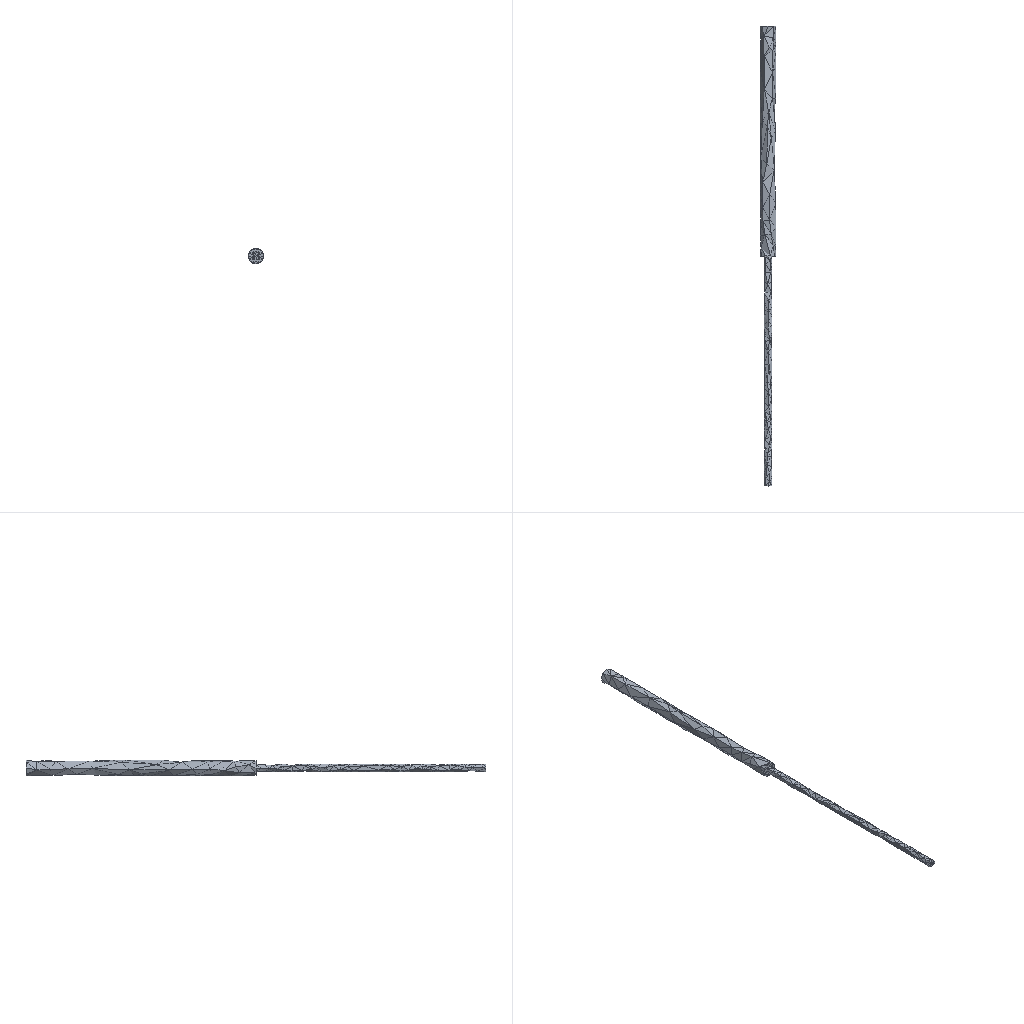Simulation study | ansys workbench
Ansys APDL input file, long lists of numbers shortened:
/batch
/config,noeldb,1     ! force off writing results to database
*get,_wallstrt,active,,time,wall
! ANSYS input file written by Workbench version 2022 R1
! File used for geometry attach: F:\ansys（分析文件汇总)\ansys有限元题目分析\1_files\dp0\SYS-1\DM\SYS-1.scdoc
/title,1--____ (B5)
! ****** Begin Custom Load Command Snippet ******
/COM, ACT Extensions:
/COM,     LSDYNA, 2021.1
/COM,
! ****** End   Custom Load Command Snippet ******
*DIM,_wb_ProjectScratch_dir,string,248
_wb_ProjectScratch_dir(1) = 'F:\ansys（分析文件汇总)\ansys有限元题目分析\_ProjectScratch\Scr897A\'
*DIM,_wb_SolverFiles_dir,string,248
_wb_SolverFiles_dir(1) = 'F:\ansys（分析文件汇总)\ansys有限元题目分析\1_files\dp0\SYS-1\MECH\'
*DIM,_wb_userfiles_dir,string,248
_wb_userfiles_dir(1) = 'F:\ansys（分析文件汇总)\ansys有限元题目分析\1_files\user_files\'
/com,--- Data in consistent NMM units. See Solving Units in the help system for more information.
/units,MPA
/nopr
/wb,file,start              !  signify a WB generated input file
/prep7
! Turn off shape checking because checks already performed inside WB mesher.
! See help system for more information.
SHPP,OFF,,NOWARN
/nolist
etcon,set             ! allow ANSYS to choose best KEYOP's for 180x elements, resets any applicable keyopt to MAPDL defaults
/com,*********** Nodes for the whole assembly ***********
nblock,3,,134372
(1i9,3e20.9e3)
        1    -5.000000000E+01     4.405700000E+02    -2.832769449E-14
! (122156 more lines like these left out)
-1
/com,*********** Nodes for all Remote Points ***********
nblock,3
(1i9,3e20.9e3)
   122158     1.673250921E-03     0.000000000E+00     1.798580280E-16
   122159    -8.638767374E-16     4.405699968E+02     2.339666164E-16
   122160     1.382202767E-15     9.615300298E+02     2.159691824E-16
-1
/wb,elem,start            !  set before creation of elements
/com,*********** Elements for Body 1 "SYS-1\__" ***********
et,1,187
eblock,19,solid,,70267
(19i9)
        1        1        1        1        0        0        0        0       10        0        1     9167     9394    19171    19168    69793    71048    69798    69797
! (140533 more lines like these left out)
-1
/wb,elem,end               !  done creating elements
/com,*********** Send User Defined Coordinate System(s) ***********
csys,0
toffst,273.15,  ! Temperature offset from absolute zero
/com,*********** Set Reference Temperature ***********
tref,22.
/wb,mat,start              !  starting to send materials
/com,*********** Send Materials ***********
Temperature = 'TEMP' ! Temperature
MP,DENS,1,7.85e-09,	! tonne mm^-3
MP,ALPX,1,1.2e-05,	! C^-1
MP,C,1,434000000,	! mm^2 s^-2 C^-1
MP,KXX,1,60.5,	! tonne mm s^-3 C^-1
MP,RSVX,1,0.00017,	! ohm mm
MP,EX,1,200000,	! tonne s^-2 mm^-1
MP,NUXY,1,0.3,
MP,MURX,1,10000,
/wb,mat,end                !  done sending materials
!************************* Model Summary ********************
!SYS-1\__,	结构钢,	matid,	1
!************************* End Model Summary ********************
! get the diagonal of the bounding box. Needed later for other things
*get,_xmin,node,,mnloc,x
*get,_ymin,node,,mnloc,y
*get,_zmin,node,,mnloc,z
*get,_xmax,node,,mxloc,x
*get,_ymax,node,,mxloc,y
*get,_zmax,node,,mxloc,z
_ASMDIAG=(_xmax-_xmin)*(_xmax-_xmin)+(_ymax-_ymin)*(_ymax-_ymin)+(_zmax-_zmin)*(_zmax-_zmin)
_ASMDIAG=SQRT(_ASMDIAG)
/wb,contact,start          !  starting to send contact
/wb,contact,end            !  done creating contacts
/golist
/wb,load,start             !  starting to send loads
/com,*********** Fixed Supports ***********
CMBLOCK,_FIXEDSU,NODE,     1223
(8i10)
        64        65        66        67        68        69        70        71
! (152 more lines like these left out)
cmsel,s,_FIXEDSU
d,all,all
nsel,all
/com,*********** Create Remote Point "内部远程点" ***********
! -------- Remote Point Used by "力矩" --------
*set,tid,3
*set,cid,2
et,cid,177
et,tid,170
keyo,tid,2,1               ! Don't fix the pilot node
keyo,tid,4,111111
keyo,cid,12,5              ! Bonded Contact
keyo,cid,4,1               ! Deformable RBE3 style load
keyo,cid,2,2               ! MPC style contact
eblock,10,,,76
(15i9)
    97369        2        2        2        0      204      203    20501
! (75 more lines like these left out)
-1
*set,_npilot,122158
_npilot33=_npilot
type,tid
mat ,cid
real,cid
tshape,pilo
en,97445,_npilot
tshape
/com,*********** Create Remote Point "内部远程点 2" ***********
! -------- Remote Point Used by "力矩 2" --------
*set,tid,5
*set,cid,4
et,cid,177
et,tid,170
keyo,tid,2,1               ! Don't fix the pilot node
keyo,tid,4,111111
keyo,cid,12,5              ! Bonded Contact
keyo,cid,4,1               ! Deformable RBE3 style load
keyo,cid,2,2               ! MPC style contact
eblock,10,,,76
(15i9)
    97446        4        4        4        0      127      128    20162
! (75 more lines like these left out)
-1
*set,_npilot,122159
_npilot36=_npilot
type,tid
mat ,cid
real,cid
tshape,pilo
en,97522,_npilot
tshape
/com,*********** Create Remote Point "内部远程点 3" ***********
! -------- Remote Point Used by "力矩 3" --------
*set,tid,7
*set,cid,6
et,cid,177
et,tid,170
keyo,tid,2,1               ! Don't fix the pilot node
keyo,tid,4,111111
keyo,cid,12,5              ! Bonded Contact
keyo,cid,4,1               ! Deformable RBE3 style load
keyo,cid,2,2               ! MPC style contact
eblock,10,,,63
(15i9)
    97523        6        6        6        0       64      126    19821
! (62 more lines like these left out)
-1
*set,_npilot,122160
_npilot39=_npilot
type,tid
mat ,cid
real,cid
tshape,pilo
en,97586,_npilot
tshape
/com,*********** Construct Moment Using Remote Attachment ***********
/com,*********** Construct Moment Using Remote Attachment ***********
/com,*********** Construct Moment Using Remote Attachment ***********
/gst,on,on
fini
*get,_numnode,node,0,count
*get,_numelem,elem,0,count
*get, _MAXELEMNUM, elem, 0, NUM, MAX
*get, _MAXNODENUM, node, 0, NUM, MAX
*get, _MAXELEMTYPE, etyp, 0, NUM, MAX
*get, _MAXREALCONST, real, 0, NUM, MAX
/go
/wb,load,end               !  done creating loads
/com,--- Number of total nodes = %_numnode%
/com,--- Number of contact elements = 215
/com,--- Number of spring elements = 0
/com,--- Number of bearing elements = 0
/com,--- Number of solid elements = 70267
/com,--- Number of condensed parts = 0
/com,--- Number of total elements = %_numelem%
*get,_wallbsol,active,,time,wall
/com,****************************************************************************
/com,*************************    SOLUTION       ********************************
/com,****************************************************************************
/solu
antype,0                   ! static analysis
_thickRatio=  1     ! Ratio of thick parts in the model
eqsl,pcg,1e-8,,,,,,1
cntr,print,1               ! print out contact info and also make no initial contact an error
dmpoption,emat,no             ! Don't combine emat file for DANSYS
dmpoption,esav,no             ! Don't combine esav file for DANSYS
nldiag,cont,iter           ! print out contact info each equilibrium iteration
rescontrol,,none                 ! Do not keep any restart files
/com,****************************************************
/com,******************* SOLVE FOR LS 1 OF 1 ****************
nsel,s,node,,122158
f,all,mx,0.
f,all,my,-22000000.
f,all,mz,0.
nsel,s,node,,122159
f,all,mx,0.
f,all,my,-36000000.
f,all,mz,0.
nsel,s,node,,122160
f,all,mx,0.
f,all,my,-14000000.
f,all,mz,0.
nsel,all
/nopr
/gopr
nsub,1,1,1
time,1.
outres,erase
outres,all,none
outres,nsol,all,
outres,rsol,all
outres,eangl,all
outres,etmp,all
outres,veng,all
outres,strs,all,
outres,epel,all,
outres,eppl,all,
outres,cont,all,
! *********** WB SOLVE COMMAND ***********
! check interactive state
*get,ANSINTER_,active,,int
*if,ANSINTER_,ne,0,then
/eof
*endif
solve
/com *************** Write FE CONNECTORS *********
CEWRITE,file,ce,,INTE
/com,****************************************************
/com,*************** FINISHED SOLVE FOR LS 1 *************
*get,_wallasol,active,,time,wall
/nopr
*get,_numnode,node,0,count
*get,_numelem,elem,0,count
*get, _MAXELEMNUM, elem, 0, NUM, MAX
*get, _MAXNODENUM, node, 0, NUM, MAX,,,INTERNAL
*get, _MAXELEMTYPE, etyp, 0, NUM, MAX
*get, _MAXREALCONST, real, 0, NUM, MAX
/gopr
*get,_PCGITER,active,,solu,cgiter
/post1
xmlo,ENCODING,ISO-8859-1
xmlo,parm
/xml,parm,xml
fini
/gopr
*get,_walldone,active,,time,wall
_preptime=(_wallbsol-_wallstrt)*3600
_solvtime=(_wallasol-_wallbsol)*3600
_posttime=(_walldone-_wallasol)*3600
_totaltim=(_walldone-_wallstrt)*3600
*get,_dlbratio,active,0,solu,dlbr
*get,_combtime,active,0,solu,comb
*get,_ssmode,active,0,solu,ssmm
*get,_ndofs,active,0,solu,ndof
*get,_sol_end_time,active,0,set,time
*if,_sol_end_time,eq,1.,then
/fclean				!clean distributed files
*endif
/com,--- Total number of nodes = %_numnode%
/com,--- Total number of elements = %_numelem%
/com,--- Element load balance ratio = %_dlbratio%
/com,--- Time to combine distributed files = %_combtime%
/com,--- Sparse memory mode = %_ssmode%
/com,--- Number of DOF = %_ndofs%
/wb,file,end               ! done with WB generated input